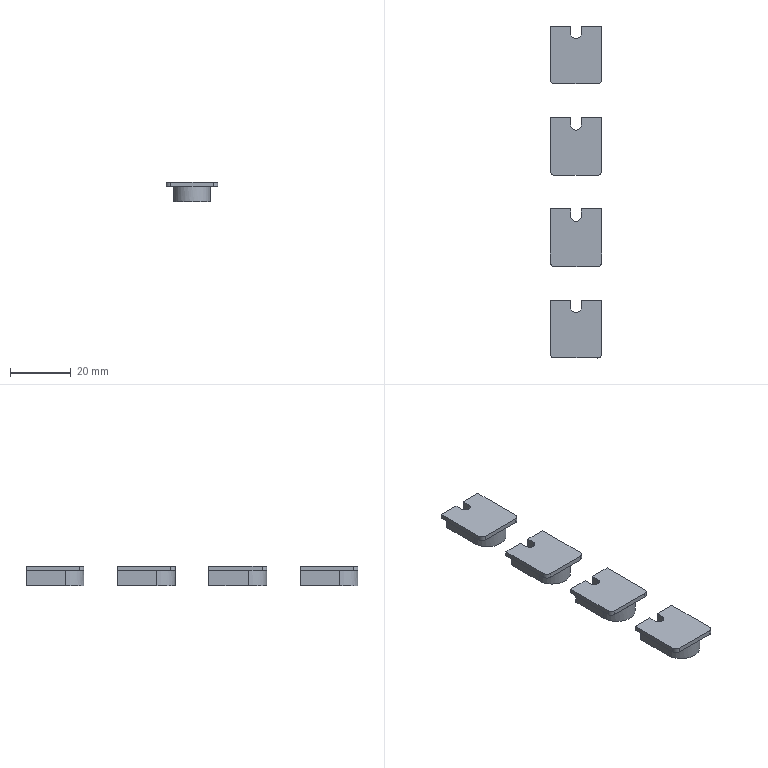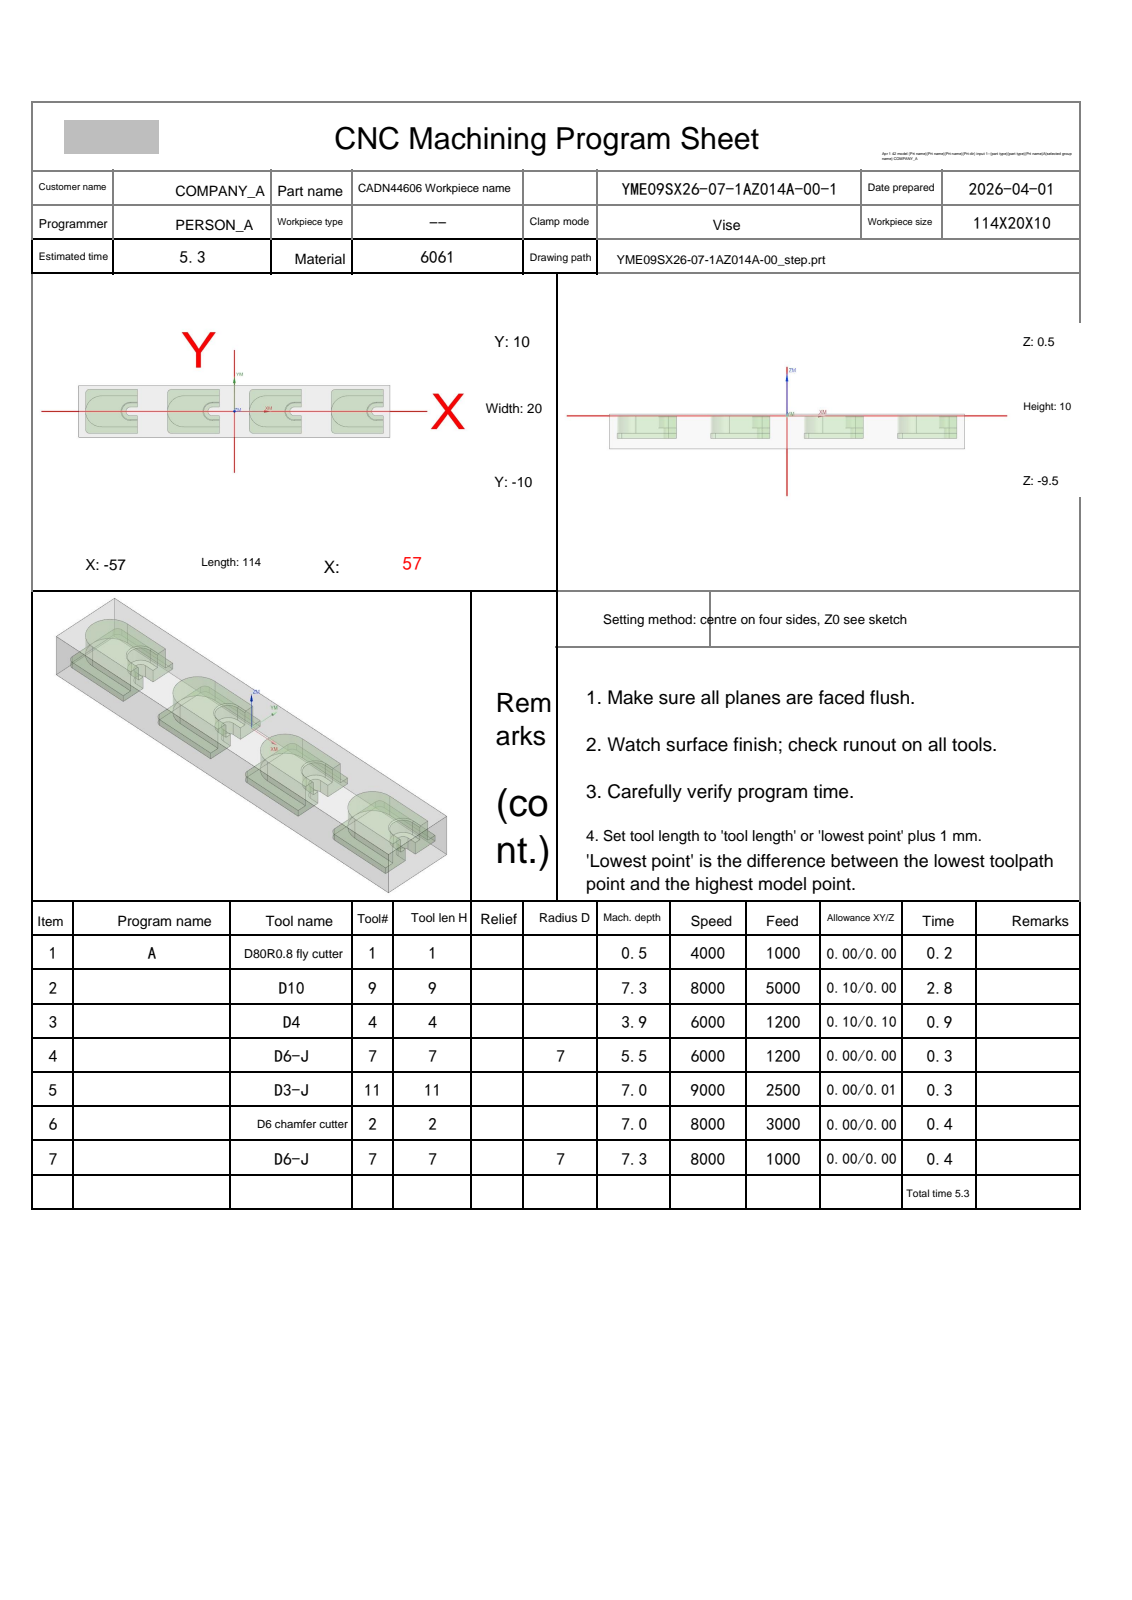NC program | NX | posted by the shop | part box 17.001 x 109 x 6.504 mm
Lines 2417 to 4321 of 4321, first 1691 of 1905 lines:
N5 T11 M06
(D3-J  D=3. R=0. H=11 ce=0.00 di=0.01)
G00 G90 G54 X-33.527 Y1.705 M03 S9000
G43 H11 Z20.
M08
Z-3.068
G01 X-33.532 Z-3.133 F2000.
X-33.547 Z-3.191
X-33.569 Y1.704 Z-3.243
X-33.598 Y1.703 Z-3.29
X-33.633 Y1.7 Z-3.332
X-33.673 Y1.696 Z-3.369
X-33.715 Y1.689 Z-3.401
X-33.758 Y1.68 Z-3.428
X-33.803 Y1.669 Z-3.451
X-33.846 Y1.654 Z-3.471
X-33.887 Y1.635 Z-3.486
X-33.925 Y1.613 Z-3.498
X-33.958 Y1.587 Z-3.508
X-33.985 Y1.555 Z-3.514
X-34.005 Y1.519 Z-3.517
X-34.017 Y1.477 Z-3.518
G02 X-35.501 Y.2 I-1.484 J.223 F2500.
G01 X-35.537
X-37.998
X-38.
G03 X-38.2 Y0.0 I0.0 J-.2
G01 X-38.13 Y-.152
X-38.097 Y-.186
X-38.053 Y-.203
X-38.005 Y-.2
X-35.489
G02 X-34.017 Y-1.477 I-.011 J-1.5
G01 X-34.002 Y-1.508 Z-3.519
X-33.974 Y-1.502 Z-3.523
X-33.936 Y-1.464 Z-3.529
X-33.89 Y-1.398 Z-3.537
X-33.84 Y-1.306 Z-3.547
X-33.787 Y-1.193 Z-3.558
X-33.735 Y-1.062 Z-3.57
X-33.687 Y-.918 Z-3.584
X-33.644 Y-.763 Z-3.598
X-33.588 Y-.467 Z-3.624
X-33.56 Y-.158 Z-3.651
Y.156 Z-3.679
X-33.588 Y.465 Z-3.706
X-33.644 Y.761 Z-3.732
X-33.687 Y.916 Z-3.746
X-33.735 Y1.061 Z-3.759
X-33.787 Y1.192 Z-3.772
X-33.84 Y1.305 Z-3.783
X-33.89 Y1.397 Z-3.792
X-33.936 Y1.464 Z-3.8
X-33.974 Y1.502 Z-3.806
X-34.002 Y1.508 Z-3.81
X-34.017 Y1.477 Z-3.811
G02 X-35.5 Y.2 I-1.483 J.223
G01 X-35.506
X-37.998
X-38.
G03 X-38.2 Y0.0 I0.0 J-.2
G01 X-38.13 Y-.152
X-38.097 Y-.186
X-38.053 Y-.203
X-38.005 Y-.2
X-35.489
G02 X-34.017 Y-1.477 I-.011 J-1.5
G01 X-34.002 Y-1.508 Z-3.813
X-33.974 Y-1.502 Z-3.816
X-33.936 Y-1.464 Z-3.822
X-33.89 Y-1.398 Z-3.83
X-33.84 Y-1.306 Z-3.84
X-33.787 Y-1.193 Z-3.851
X-33.735 Y-1.062 Z-3.864
X-33.687 Y-.918 Z-3.877
X-33.644 Y-.763 Z-3.891
X-33.588 Y-.467 Z-3.917
X-33.56 Y-.158 Z-3.944
Y.156 Z-3.972
X-33.588 Y.465 Z-3.999
X-33.644 Y.761 Z-4.025
X-33.687 Y.916 Z-4.039
X-33.735 Y1.061 Z-4.052
X-33.787 Y1.192 Z-4.065
X-33.84 Y1.305 Z-4.076
X-33.89 Y1.397 Z-4.086
X-33.936 Y1.464 Z-4.093
X-33.974 Y1.502 Z-4.099
X-34.002 Y1.508 Z-4.103
X-34.017 Y1.477 Z-4.105
G02 X-35.5 Y.2 I-1.483 J.223
G01 X-35.506
X-37.998
X-38.
G03 X-38.2 Y0.0 I0.0 J-.2
G01 X-38.13 Y-.152
X-38.097 Y-.186
X-38.053 Y-.203
X-38.005 Y-.2
X-35.489
G02 X-34.017 Y-1.477 I-.011 J-1.5
G01 X-34.002 Y-1.508 Z-4.106
X-33.974 Y-1.502 Z-4.11
X-33.936 Y-1.464 Z-4.116
X-33.89 Y-1.398 Z-4.124
X-33.84 Y-1.306 Z-4.133
X-33.787 Y-1.193 Z-4.144
X-33.735 Y-1.062 Z-4.157
X-33.687 Y-.918 Z-4.17
X-33.644 Y-.763 Z-4.184
X-33.588 Y-.467 Z-4.21
X-33.56 Y-.158 Z-4.237
Y.156 Z-4.265
X-33.588 Y.465 Z-4.292
X-33.644 Y.761 Z-4.318
X-33.687 Y.916 Z-4.332
X-33.735 Y1.061 Z-4.346
X-33.787 Y1.192 Z-4.358
X-33.84 Y1.305 Z-4.369
X-33.89 Y1.397 Z-4.379
X-33.936 Y1.464 Z-4.387
X-33.974 Y1.502 Z-4.393
X-34.002 Y1.508 Z-4.396
X-34.017 Y1.477 Z-4.398
G02 X-35.5 Y.2 I-1.483 J.223
G01 X-35.506
X-37.998
X-38.
G03 X-38.2 Y0.0 I0.0 J-.2
G01 X-38.13 Y-.152
X-38.097 Y-.186
X-38.053 Y-.203
X-38.005 Y-.2
X-35.489
G02 X-34.017 Y-1.477 I-.011 J-1.5
G01 X-34.002 Y-1.508 Z-4.399
X-33.974 Y-1.502 Z-4.403
X-33.936 Y-1.464 Z-4.409
X-33.89 Y-1.398 Z-4.417
X-33.84 Y-1.306 Z-4.426
X-33.787 Y-1.193 Z-4.438
X-33.735 Y-1.062 Z-4.45
X-33.687 Y-.918 Z-4.463
X-33.644 Y-.763 Z-4.477
X-33.588 Y-.467 Z-4.503
X-33.56 Y-.158 Z-4.531
Y.156 Z-4.558
X-33.588 Y.465 Z-4.585
X-33.644 Y.761 Z-4.612
X-33.687 Y.916 Z-4.625
X-33.735 Y1.061 Z-4.639
X-33.787 Y1.192 Z-4.651
X-33.84 Y1.305 Z-4.662
X-33.89 Y1.397 Z-4.672
X-33.936 Y1.464 Z-4.68
X-33.974 Y1.502 Z-4.686
X-34.002 Y1.508 Z-4.69
X-34.017 Y1.477 Z-4.691
G02 X-35.5 Y.2 I-1.483 J.223
G01 X-35.506
X-37.998
X-38.
G03 X-38.2 Y0.0 I0.0 J-.2
G01 X-38.13 Y-.152
X-38.097 Y-.186
X-38.053 Y-.203
X-38.005 Y-.2
X-35.489
G02 X-34.017 Y-1.477 I-.011 J-1.5
G01 X-34.002 Y-1.508 Z-4.692
X-33.974 Y-1.502 Z-4.696
X-33.936 Y-1.464 Z-4.702
X-33.89 Y-1.398 Z-4.71
X-33.84 Y-1.306 Z-4.72
X-33.787 Y-1.193 Z-4.731
X-33.735 Y-1.062 Z-4.743
X-33.687 Y-.918 Z-4.756
X-33.644 Y-.763 Z-4.77
X-33.588 Y-.467 Z-4.797
X-33.56 Y-.158 Z-4.824
Y.156 Z-4.851
X-33.588 Y.465 Z-4.878
X-33.644 Y.761 Z-4.905
X-33.687 Y.916 Z-4.919
X-33.735 Y1.061 Z-4.932
X-33.787 Y1.192 Z-4.944
X-33.84 Y1.305 Z-4.955
X-33.89 Y1.397 Z-4.965
X-33.936 Y1.464 Z-4.973
X-33.974 Y1.502 Z-4.979
X-34.002 Y1.508 Z-4.983
X-34.017 Y1.477 Z-4.984
G02 X-35.5 Y.2 I-1.483 J.223
G01 X-35.506
X-37.998
X-38.
G03 X-38.2 Y0.0 I0.0 J-.2
G01 X-38.13 Y-.152
X-38.097 Y-.186
X-38.053 Y-.203
X-38.005 Y-.2
X-35.489
G02 X-34.017 Y-1.477 I-.011 J-1.5
G01 X-34.002 Y-1.508 Z-4.985
X-33.974 Y-1.502 Z-4.989
X-33.936 Y-1.464 Z-4.995
X-33.89 Y-1.398 Z-5.003
X-33.84 Y-1.306 Z-5.013
X-33.787 Y-1.193 Z-5.024
X-33.735 Y-1.062 Z-5.036
X-33.687 Y-.918 Z-5.05
X-33.644 Y-.763 Z-5.063
X-33.588 Y-.467 Z-5.09
X-33.56 Y-.158 Z-5.117
Y.156 Z-5.144
X-33.588 Y.465 Z-5.172
X-33.644 Y.761 Z-5.198
X-33.687 Y.916 Z-5.212
X-33.735 Y1.061 Z-5.225
X-33.787 Y1.192 Z-5.237
X-33.84 Y1.305 Z-5.249
X-33.89 Y1.397 Z-5.258
X-33.936 Y1.464 Z-5.266
X-33.974 Y1.502 Z-5.272
X-34.002 Y1.508 Z-5.276
X-34.017 Y1.477 Z-5.277
G02 X-35.5 Y.2 I-1.483 J.223
G01 X-35.506
X-37.998
X-38.
G03 X-38.2 Y0.0 I0.0 J-.2
G01 X-38.13 Y-.152
X-38.097 Y-.186
X-38.053 Y-.203
X-38.005 Y-.2
X-35.489
G02 X-34.017 Y-1.477 I-.011 J-1.5
G01 X-34.002 Y-1.508 Z-5.279
X-33.974 Y-1.502 Z-5.282
X-33.936 Y-1.464 Z-5.288
X-33.89 Y-1.398 Z-5.296
X-33.84 Y-1.306 Z-5.306
X-33.787 Y-1.193 Z-5.317
X-33.735 Y-1.062 Z-5.329
X-33.687 Y-.918 Z-5.343
X-33.644 Y-.763 Z-5.357
X-33.588 Y-.467 Z-5.383
X-33.56 Y-.158 Z-5.41
Y.156 Z-5.438
X-33.588 Y.465 Z-5.465
X-33.644 Y.761 Z-5.491
X-33.687 Y.916 Z-5.505
X-33.735 Y1.061 Z-5.518
X-33.787 Y1.192 Z-5.531
X-33.84 Y1.305 Z-5.542
X-33.89 Y1.397 Z-5.551
X-33.936 Y1.464 Z-5.559
X-33.974 Y1.502 Z-5.565
X-34.002 Y1.508 Z-5.569
X-34.017 Y1.477 Z-5.57
G02 X-35.5 Y.2 I-1.483 J.223
G01 X-35.506
X-37.998
X-38.
G03 X-38.2 Y0.0 I0.0 J-.2
G01 X-38.13 Y-.152
X-38.097 Y-.186
X-38.053 Y-.203
X-38.005 Y-.2
X-35.489
G02 X-34.017 Y-1.477 I-.011 J-1.5
G01 X-34.002 Y-1.508 Z-5.572
X-33.974 Y-1.502 Z-5.576
X-33.936 Y-1.464 Z-5.582
X-33.89 Y-1.398 Z-5.589
X-33.84 Y-1.306 Z-5.599
X-33.787 Y-1.193 Z-5.61
X-33.735 Y-1.062 Z-5.623
X-33.687 Y-.918 Z-5.636
X-33.644 Y-.763 Z-5.65
X-33.588 Y-.467 Z-5.676
X-33.56 Y-.158 Z-5.703
Y.156 Z-5.731
X-33.588 Y.465 Z-5.758
X-33.644 Y.761 Z-5.784
X-33.687 Y.916 Z-5.798
X-33.735 Y1.061 Z-5.811
X-33.787 Y1.192 Z-5.824
X-33.84 Y1.305 Z-5.835
X-33.89 Y1.397 Z-5.845
X-33.936 Y1.464 Z-5.853
X-33.974 Y1.502 Z-5.859
X-34.002 Y1.508 Z-5.862
X-34.017 Y1.477 Z-5.864
G02 X-35.5 Y.2 I-1.483 J.223
G01 X-35.506
X-37.998
X-38.
G03 X-38.2 Y0.0 I0.0 J-.2
G01 X-38.13 Y-.152
X-38.097 Y-.186
X-38.053 Y-.203
X-38.005 Y-.2
X-35.489
G02 X-34.017 Y-1.477 I-.011 J-1.5
G01 X-34.002 Y-1.508 Z-5.865
X-33.974 Y-1.502 Z-5.869
X-33.936 Y-1.464 Z-5.875
X-33.89 Y-1.398 Z-5.883
X-33.84 Y-1.306 Z-5.892
X-33.787 Y-1.193 Z-5.903
X-33.735 Y-1.062 Z-5.916
X-33.687 Y-.918 Z-5.929
X-33.644 Y-.763 Z-5.943
X-33.588 Y-.467 Z-5.969
X-33.56 Y-.158 Z-5.996
Y.156 Z-6.024
X-33.588 Y.465 Z-6.051
X-33.644 Y.761 Z-6.077
X-33.687 Y.916 Z-6.091
X-33.735 Y1.061 Z-6.105
X-33.787 Y1.192 Z-6.117
X-33.84 Y1.305 Z-6.128
X-33.89 Y1.397 Z-6.138
X-33.936 Y1.464 Z-6.146
X-33.974 Y1.502 Z-6.152
X-34.002 Y1.508 Z-6.156
X-34.017 Y1.477 Z-6.157
G02 X-35.5 Y.2 I-1.483 J.223
G01 X-35.506
X-37.998
X-38.
G03 X-38.2 Y0.0 I0.0 J-.2
G01 X-38.13 Y-.152
X-38.097 Y-.186
X-38.053 Y-.203
X-38.005 Y-.2
X-35.489
G02 X-34.017 Y-1.477 I-.011 J-1.5
G01 X-34.002 Y-1.508 Z-6.158
X-33.974 Y-1.502 Z-6.162
X-33.936 Y-1.464 Z-6.168
X-33.89 Y-1.398 Z-6.176
X-33.84 Y-1.306 Z-6.186
X-33.787 Y-1.193 Z-6.197
X-33.735 Y-1.062 Z-6.209
X-33.687 Y-.918 Z-6.222
X-33.644 Y-.763 Z-6.236
X-33.588 Y-.467 Z-6.263
X-33.56 Y-.158 Z-6.29
Y.156 Z-6.317
X-33.588 Y.465 Z-6.344
X-33.644 Y.761 Z-6.371
X-33.687 Y.916 Z-6.385
X-33.735 Y1.061 Z-6.398
X-33.787 Y1.192 Z-6.41
X-33.84 Y1.305 Z-6.421
X-33.89 Y1.397 Z-6.431
X-33.936 Y1.464 Z-6.439
X-33.974 Y1.502 Z-6.445
X-34.002 Y1.508 Z-6.449
X-34.017 Y1.477 Z-6.45
G02 X-35.5 Y.2 I-1.483 J.223
G01 X-35.506
X-37.998
X-38.
G03 X-38.2 Y0.0 I0.0 J-.2
G01 X-38.13 Y-.152
X-38.097 Y-.186
X-38.053 Y-.203
X-38.005 Y-.2
X-35.489
G02 X-34.017 Y-1.477 I-.011 J-1.5
G01 X-33.986 Y-1.515 Z-6.449
X-33.947 Y-1.546 Z-6.445
X-33.902 Y-1.573 Z-6.438
X-33.852 Y-1.596 Z-6.427
X-33.799 Y-1.614 Z-6.413
X-33.744 Y-1.628 Z-6.395
X-33.689 Y-1.64 Z-6.373
X-33.634 Y-1.648 Z-6.346
X-33.582 Y-1.654 Z-6.314
X-33.535 Y-1.658 Z-6.277
X-33.492 Y-1.66 Z-6.234
X-33.456 Y-1.661 Z-6.185
X-33.429 Z-6.13
X-33.412 Z-6.068
X-33.406 Z-6.
G00 Z20.
X-3.527 Y1.705
Z-3.068
G01 X-3.532 Z-3.133 F2000.
X-3.547 Z-3.191
X-3.569 Y1.704 Z-3.243
X-3.598 Y1.703 Z-3.29
X-3.633 Y1.7 Z-3.332
X-3.673 Y1.696 Z-3.369
X-3.715 Y1.689 Z-3.401
X-3.758 Y1.68 Z-3.428
X-3.803 Y1.669 Z-3.451
X-3.846 Y1.654 Z-3.471
X-3.887 Y1.635 Z-3.486
X-3.925 Y1.613 Z-3.498
X-3.958 Y1.587 Z-3.508
X-3.985 Y1.555 Z-3.514
X-4.005 Y1.519 Z-3.517
X-4.017 Y1.477 Z-3.518
G02 X-5.493 Y.2 I-1.483 J.223 F2500.
G01 X-7.998
X-8.
G03 X-8.2 Y0.0 I0.0 J-.2
X-8. Y-.2 I.2 J0.0
G01 X-7.998
X-5.489
G02 X-4.017 Y-1.477 I-.011 J-1.5
G01 X-4.002 Y-1.507 Z-3.519
X-3.975 Y-1.499 Z-3.523
X-3.937 Y-1.457 Z-3.529
X-3.892 Y-1.386 Z-3.537
X-3.842 Y-1.289 Z-3.547
X-3.791 Y-1.171 Z-3.558
X-3.739 Y-1.035 Z-3.57
X-3.691 Y-.886 Z-3.584
X-3.649 Y-.728 Z-3.598
X-3.593 Y-.43 Z-3.624
X-3.565 Y-.122 Z-3.651
X-3.564 Y.187 Z-3.679
X-3.591 Y.491 Z-3.706
X-3.647 Y.781 Z-3.732
X-3.689 Y.932 Z-3.746
X-3.737 Y1.074 Z-3.759
X-3.789 Y1.202 Z-3.772
X-3.841 Y1.312 Z-3.783
X-3.891 Y1.402 Z-3.792
X-3.936 Y1.467 Z-3.8
X-3.974 Y1.503 Z-3.806
X-4.002 Y1.508 Z-3.81
X-4.017 Y1.477 Z-3.811
G02 X-5.493 Y.2 I-1.483 J.223
G01 X-7.998
X-8.
G03 X-8.2 Y0.0 I0.0 J-.2
X-8. Y-.2 I.2 J0.0
G01 X-7.998
X-5.489
G02 X-4.017 Y-1.477 I-.011 J-1.5
G01 X-4.002 Y-1.507 Z-3.813
X-3.975 Y-1.499 Z-3.816
X-3.937 Y-1.457 Z-3.822
X-3.892 Y-1.386 Z-3.83
X-3.842 Y-1.289 Z-3.84
X-3.791 Y-1.171 Z-3.851
X-3.739 Y-1.035 Z-3.864
X-3.691 Y-.886 Z-3.877
X-3.649 Y-.728 Z-3.891
X-3.593 Y-.43 Z-3.917
X-3.565 Y-.122 Z-3.944
X-3.564 Y.187 Z-3.972
X-3.591 Y.491 Z-3.999
X-3.647 Y.781 Z-4.025
X-3.689 Y.932 Z-4.039
X-3.737 Y1.074 Z-4.052
X-3.789 Y1.202 Z-4.065
X-3.841 Y1.312 Z-4.076
X-3.891 Y1.402 Z-4.086
X-3.936 Y1.467 Z-4.093
X-3.974 Y1.503 Z-4.099
X-4.002 Y1.508 Z-4.103
X-4.017 Y1.477 Z-4.105
G02 X-5.493 Y.2 I-1.483 J.223
G01 X-7.998
X-8.
G03 X-8.2 Y0.0 I0.0 J-.2
X-8. Y-.2 I.2 J0.0
G01 X-7.998
X-5.489
G02 X-4.017 Y-1.477 I-.011 J-1.5
G01 X-4.002 Y-1.507 Z-4.106
X-3.975 Y-1.499 Z-4.11
X-3.937 Y-1.457 Z-4.116
X-3.892 Y-1.386 Z-4.124
X-3.842 Y-1.289 Z-4.133
X-3.791 Y-1.171 Z-4.144
X-3.739 Y-1.035 Z-4.157
X-3.691 Y-.886 Z-4.17
X-3.649 Y-.728 Z-4.184
X-3.593 Y-.43 Z-4.21
X-3.565 Y-.122 Z-4.237
X-3.564 Y.187 Z-4.265
X-3.591 Y.491 Z-4.292
X-3.647 Y.781 Z-4.318
X-3.689 Y.932 Z-4.332
X-3.737 Y1.074 Z-4.346
X-3.789 Y1.202 Z-4.358
X-3.841 Y1.312 Z-4.369
X-3.891 Y1.402 Z-4.379
X-3.936 Y1.467 Z-4.387
X-3.974 Y1.503 Z-4.393
X-4.002 Y1.508 Z-4.396
X-4.017 Y1.477 Z-4.398
G02 X-5.493 Y.2 I-1.483 J.223
G01 X-7.998
X-8.
G03 X-8.2 Y0.0 I0.0 J-.2
X-8. Y-.2 I.2 J0.0
G01 X-7.998
X-5.489
G02 X-4.017 Y-1.477 I-.011 J-1.5
G01 X-4.002 Y-1.507 Z-4.399
X-3.975 Y-1.499 Z-4.403
X-3.937 Y-1.457 Z-4.409
X-3.892 Y-1.386 Z-4.417
X-3.842 Y-1.289 Z-4.426
X-3.791 Y-1.171 Z-4.438
X-3.739 Y-1.035 Z-4.45
X-3.691 Y-.886 Z-4.463
X-3.649 Y-.728 Z-4.477
X-3.593 Y-.43 Z-4.503
X-3.565 Y-.122 Z-4.531
X-3.564 Y.187 Z-4.558
X-3.591 Y.491 Z-4.585
X-3.647 Y.781 Z-4.612
X-3.689 Y.932 Z-4.625
X-3.737 Y1.074 Z-4.639
X-3.789 Y1.202 Z-4.651
X-3.841 Y1.312 Z-4.662
X-3.891 Y1.402 Z-4.672
X-3.936 Y1.467 Z-4.68
X-3.974 Y1.503 Z-4.686
X-4.002 Y1.508 Z-4.69
X-4.017 Y1.477 Z-4.691
G02 X-5.493 Y.2 I-1.483 J.223
G01 X-7.998
X-8.
G03 X-8.2 Y0.0 I0.0 J-.2
X-8. Y-.2 I.2 J0.0
G01 X-7.998
X-5.489
G02 X-4.017 Y-1.477 I-.011 J-1.5
G01 X-4.002 Y-1.507 Z-4.692
X-3.975 Y-1.499 Z-4.696
X-3.937 Y-1.457 Z-4.702
X-3.892 Y-1.386 Z-4.71
X-3.842 Y-1.289 Z-4.72
X-3.791 Y-1.171 Z-4.731
X-3.739 Y-1.035 Z-4.743
X-3.691 Y-.886 Z-4.756
X-3.649 Y-.728 Z-4.77
X-3.593 Y-.43 Z-4.797
X-3.565 Y-.122 Z-4.824
X-3.564 Y.187 Z-4.851
X-3.591 Y.491 Z-4.878
X-3.647 Y.781 Z-4.905
X-3.689 Y.932 Z-4.919
X-3.737 Y1.074 Z-4.932
X-3.789 Y1.202 Z-4.944
X-3.841 Y1.312 Z-4.955
X-3.891 Y1.402 Z-4.965
X-3.936 Y1.467 Z-4.973
X-3.974 Y1.503 Z-4.979
X-4.002 Y1.508 Z-4.983
X-4.017 Y1.477 Z-4.984
G02 X-5.493 Y.2 I-1.483 J.223
G01 X-7.998
X-8.
G03 X-8.2 Y0.0 I0.0 J-.2
X-8. Y-.2 I.2 J0.0
G01 X-7.998
X-5.489
G02 X-4.017 Y-1.477 I-.011 J-1.5
G01 X-4.002 Y-1.507 Z-4.985
X-3.975 Y-1.499 Z-4.989
X-3.937 Y-1.457 Z-4.995
X-3.892 Y-1.386 Z-5.003
X-3.842 Y-1.289 Z-5.013
X-3.791 Y-1.171 Z-5.024
X-3.739 Y-1.035 Z-5.036
X-3.691 Y-.886 Z-5.05
X-3.649 Y-.728 Z-5.063
X-3.593 Y-.43 Z-5.09
X-3.565 Y-.122 Z-5.117
X-3.564 Y.187 Z-5.144
X-3.591 Y.491 Z-5.172
X-3.647 Y.781 Z-5.198
X-3.689 Y.932 Z-5.212
X-3.737 Y1.074 Z-5.225
X-3.789 Y1.202 Z-5.237
X-3.841 Y1.312 Z-5.249
X-3.891 Y1.402 Z-5.258
X-3.936 Y1.467 Z-5.266
X-3.974 Y1.503 Z-5.272
X-4.002 Y1.508 Z-5.276
X-4.017 Y1.477 Z-5.277
G02 X-5.493 Y.2 I-1.483 J.223
G01 X-7.998
X-8.
G03 X-8.2 Y0.0 I0.0 J-.2
X-8. Y-.2 I.2 J0.0
G01 X-7.998
X-5.489
G02 X-4.017 Y-1.477 I-.011 J-1.5
G01 X-4.002 Y-1.507 Z-5.279
X-3.975 Y-1.499 Z-5.282
X-3.937 Y-1.457 Z-5.288
X-3.892 Y-1.386 Z-5.296
X-3.842 Y-1.289 Z-5.306
X-3.791 Y-1.171 Z-5.317
X-3.739 Y-1.035 Z-5.329
X-3.691 Y-.886 Z-5.343
X-3.649 Y-.728 Z-5.357
X-3.593 Y-.43 Z-5.383
X-3.565 Y-.122 Z-5.41
X-3.564 Y.187 Z-5.438
X-3.591 Y.491 Z-5.465
X-3.647 Y.781 Z-5.491
X-3.689 Y.932 Z-5.505
X-3.737 Y1.074 Z-5.518
X-3.789 Y1.202 Z-5.531
X-3.841 Y1.312 Z-5.542
X-3.891 Y1.402 Z-5.551
X-3.936 Y1.467 Z-5.559
X-3.974 Y1.503 Z-5.565
X-4.002 Y1.508 Z-5.569
X-4.017 Y1.477 Z-5.57
G02 X-5.493 Y.2 I-1.483 J.223
G01 X-7.998
X-8.
G03 X-8.2 Y0.0 I0.0 J-.2
X-8. Y-.2 I.2 J0.0
G01 X-7.998
X-5.489
G02 X-4.017 Y-1.477 I-.011 J-1.5
G01 X-4.002 Y-1.507 Z-5.572
X-3.975 Y-1.499 Z-5.576
X-3.937 Y-1.457 Z-5.582
X-3.892 Y-1.386 Z-5.589
X-3.842 Y-1.289 Z-5.599
X-3.791 Y-1.171 Z-5.61
X-3.739 Y-1.035 Z-5.623
X-3.691 Y-.886 Z-5.636
X-3.649 Y-.728 Z-5.65
X-3.593 Y-.43 Z-5.676
X-3.565 Y-.122 Z-5.703
X-3.564 Y.187 Z-5.731
X-3.591 Y.491 Z-5.758
X-3.647 Y.781 Z-5.784
X-3.689 Y.932 Z-5.798
X-3.737 Y1.074 Z-5.811
X-3.789 Y1.202 Z-5.824
X-3.841 Y1.312 Z-5.835
X-3.891 Y1.402 Z-5.845
X-3.936 Y1.467 Z-5.853
X-3.974 Y1.503 Z-5.859
X-4.002 Y1.508 Z-5.862
X-4.017 Y1.477 Z-5.864
G02 X-5.493 Y.2 I-1.483 J.223
G01 X-7.998
X-8.
G03 X-8.2 Y0.0 I0.0 J-.2
X-8. Y-.2 I.2 J0.0
G01 X-7.998
X-5.489
G02 X-4.017 Y-1.477 I-.011 J-1.5
G01 X-4.002 Y-1.507 Z-5.865
X-3.975 Y-1.499 Z-5.869
X-3.937 Y-1.457 Z-5.875
X-3.892 Y-1.386 Z-5.883
X-3.842 Y-1.289 Z-5.892
X-3.791 Y-1.171 Z-5.903
X-3.739 Y-1.035 Z-5.916
X-3.691 Y-.886 Z-5.929
X-3.649 Y-.728 Z-5.943
X-3.593 Y-.43 Z-5.969
X-3.565 Y-.122 Z-5.996
X-3.564 Y.187 Z-6.024
X-3.591 Y.491 Z-6.051
X-3.647 Y.781 Z-6.077
X-3.689 Y.932 Z-6.091
X-3.737 Y1.074 Z-6.105
X-3.789 Y1.202 Z-6.117
X-3.841 Y1.312 Z-6.128
X-3.891 Y1.402 Z-6.138
X-3.936 Y1.467 Z-6.146
X-3.974 Y1.503 Z-6.152
X-4.002 Y1.508 Z-6.156
X-4.017 Y1.477 Z-6.157
G02 X-5.493 Y.2 I-1.483 J.223
G01 X-7.998
X-8.
G03 X-8.2 Y0.0 I0.0 J-.2
X-8. Y-.2 I.2 J0.0
G01 X-7.998
X-5.489
G02 X-4.017 Y-1.477 I-.011 J-1.5
G01 X-4.002 Y-1.507 Z-6.158
X-3.975 Y-1.499 Z-6.162
X-3.937 Y-1.457 Z-6.168
X-3.892 Y-1.386 Z-6.176
X-3.842 Y-1.289 Z-6.186
X-3.791 Y-1.171 Z-6.197
X-3.739 Y-1.035 Z-6.209
X-3.691 Y-.886 Z-6.222
X-3.649 Y-.728 Z-6.236
X-3.593 Y-.43 Z-6.263
X-3.565 Y-.122 Z-6.29
X-3.564 Y.187 Z-6.317
X-3.591 Y.491 Z-6.344
X-3.647 Y.781 Z-6.371
X-3.689 Y.932 Z-6.385
X-3.737 Y1.074 Z-6.398
X-3.789 Y1.202 Z-6.41
X-3.841 Y1.312 Z-6.421
X-3.891 Y1.402 Z-6.431
X-3.936 Y1.467 Z-6.439
X-3.974 Y1.503 Z-6.445
X-4.002 Y1.508 Z-6.449
X-4.017 Y1.477 Z-6.45
G02 X-5.493 Y.2 I-1.483 J.223
G01 X-7.998
X-8.
G03 X-8.2 Y0.0 I0.0 J-.2
X-8. Y-.2 I.2 J0.0
G01 X-7.998
X-5.489
G02 X-4.017 Y-1.477 I-.011 J-1.5
G01 X-3.986 Y-1.514 Z-6.449
X-3.948 Y-1.543 Z-6.445
X-3.903 Y-1.566 Z-6.438
X-3.854 Y-1.583 Z-6.427
X-3.802 Y-1.595 Z-6.413
X-3.748 Y-1.603 Z-6.395
X-3.693 Y-1.607 Z-6.373
X-3.64 Y-1.608 Z-6.346
X-3.589 Y-1.607 Z-6.314
X-3.542 Y-1.604 Z-6.277
X-3.501 Y-1.6 Z-6.234
X-3.466 Y-1.596 Z-6.185
X-3.439 Y-1.592 Z-6.13
X-3.422 Y-1.589 Z-6.068
X-3.416 Y-1.588 Z-6.
G00 Z20.
X26.473 Y1.705
Z-3.068
G01 X26.468 Z-3.133 F2000.
X26.453 Z-3.191
X26.431 Y1.704 Z-3.243
X26.402 Y1.703 Z-3.29
X26.367 Y1.7 Z-3.332
X26.327 Y1.696 Z-3.369
X26.285 Y1.689 Z-3.401
X26.242 Y1.68 Z-3.428
X26.197 Y1.669 Z-3.451
X26.154 Y1.654 Z-3.471
X26.113 Y1.635 Z-3.486
X26.075 Y1.613 Z-3.498
X26.042 Y1.587 Z-3.508
X26.015 Y1.555 Z-3.514
X25.995 Y1.519 Z-3.517
X25.983 Y1.477 Z-3.518
G02 X24.507 Y.2 I-1.483 J.223 F2500.
G01 X22.002
X22.
G03 X21.8 Y0.0 I0.0 J-.2
X22. Y-.2 I.2 J0.0
G01 X22.002
X24.511
G02 X25.983 Y-1.477 I-.011 J-1.5
G01 X25.998 Y-1.507 Z-3.519
X26.025 Y-1.499 Z-3.523
X26.063 Y-1.457 Z-3.529
X26.108 Y-1.386 Z-3.537
X26.158 Y-1.289 Z-3.547
X26.209 Y-1.171 Z-3.558
X26.261 Y-1.035 Z-3.57
X26.309 Y-.886 Z-3.584
X26.351 Y-.728 Z-3.598
X26.407 Y-.43 Z-3.624
X26.435 Y-.122 Z-3.651
X26.436 Y.187 Z-3.679
X26.409 Y.491 Z-3.706
X26.353 Y.781 Z-3.732
X26.311 Y.932 Z-3.746
X26.263 Y1.074 Z-3.759
X26.211 Y1.202 Z-3.772
X26.159 Y1.312 Z-3.783
X26.109 Y1.402 Z-3.792
X26.064 Y1.467 Z-3.8
X26.026 Y1.503 Z-3.806
X25.998 Y1.508 Z-3.81
X25.983 Y1.477 Z-3.811
G02 X24.507 Y.2 I-1.483 J.223
G01 X22.002
X22.
G03 X21.8 Y0.0 I0.0 J-.2
X22. Y-.2 I.2 J0.0
G01 X22.002
X24.511
G02 X25.983 Y-1.477 I-.011 J-1.5
G01 X25.998 Y-1.507 Z-3.813
X26.025 Y-1.499 Z-3.816
X26.063 Y-1.457 Z-3.822
X26.108 Y-1.386 Z-3.83
X26.158 Y-1.289 Z-3.84
X26.209 Y-1.171 Z-3.851
X26.261 Y-1.035 Z-3.864
X26.309 Y-.886 Z-3.877
X26.351 Y-.728 Z-3.891
X26.407 Y-.43 Z-3.917
X26.435 Y-.122 Z-3.944
X26.436 Y.187 Z-3.972
X26.409 Y.491 Z-3.999
X26.353 Y.781 Z-4.025
X26.311 Y.932 Z-4.039
X26.263 Y1.074 Z-4.052
X26.211 Y1.202 Z-4.065
X26.159 Y1.312 Z-4.076
X26.109 Y1.402 Z-4.086
X26.064 Y1.467 Z-4.093
X26.026 Y1.503 Z-4.099
X25.998 Y1.508 Z-4.103
X25.983 Y1.477 Z-4.105
G02 X24.507 Y.2 I-1.483 J.223
G01 X22.002
X22.
G03 X21.8 Y0.0 I0.0 J-.2
X22. Y-.2 I.2 J0.0
G01 X22.002
X24.511
G02 X25.983 Y-1.477 I-.011 J-1.5
G01 X25.998 Y-1.507 Z-4.106
X26.025 Y-1.499 Z-4.11
X26.063 Y-1.457 Z-4.116
X26.108 Y-1.386 Z-4.124
X26.158 Y-1.289 Z-4.133
X26.209 Y-1.171 Z-4.144
X26.261 Y-1.035 Z-4.157
X26.309 Y-.886 Z-4.17
X26.351 Y-.728 Z-4.184
X26.407 Y-.43 Z-4.21
X26.435 Y-.122 Z-4.237
X26.436 Y.187 Z-4.265
X26.409 Y.491 Z-4.292
X26.353 Y.781 Z-4.318
X26.311 Y.932 Z-4.332
X26.263 Y1.074 Z-4.346
X26.211 Y1.202 Z-4.358
X26.159 Y1.312 Z-4.369
X26.109 Y1.402 Z-4.379
X26.064 Y1.467 Z-4.387
X26.026 Y1.503 Z-4.393
X25.998 Y1.508 Z-4.396
X25.983 Y1.477 Z-4.398
G02 X24.507 Y.2 I-1.483 J.223
G01 X22.002
X22.
G03 X21.8 Y0.0 I0.0 J-.2
X22. Y-.2 I.2 J0.0
G01 X22.002
X24.511
G02 X25.983 Y-1.477 I-.011 J-1.5
G01 X25.998 Y-1.507 Z-4.399
X26.025 Y-1.499 Z-4.403
X26.063 Y-1.457 Z-4.409
X26.108 Y-1.386 Z-4.417
X26.158 Y-1.289 Z-4.426
X26.209 Y-1.171 Z-4.438
X26.261 Y-1.035 Z-4.45
X26.309 Y-.886 Z-4.463
X26.351 Y-.728 Z-4.477
X26.407 Y-.43 Z-4.503
X26.435 Y-.122 Z-4.531
X26.436 Y.187 Z-4.558
X26.409 Y.491 Z-4.585
X26.353 Y.781 Z-4.612
X26.311 Y.932 Z-4.625
X26.263 Y1.074 Z-4.639
X26.211 Y1.202 Z-4.651
X26.159 Y1.312 Z-4.662
X26.109 Y1.402 Z-4.672
X26.064 Y1.467 Z-4.68
X26.026 Y1.503 Z-4.686
X25.998 Y1.508 Z-4.69
X25.983 Y1.477 Z-4.691
G02 X24.507 Y.2 I-1.483 J.223
G01 X22.002
X22.
G03 X21.8 Y0.0 I0.0 J-.2
X22. Y-.2 I.2 J0.0
G01 X22.002
X24.511
G02 X25.983 Y-1.477 I-.011 J-1.5
G01 X25.998 Y-1.507 Z-4.692
X26.025 Y-1.499 Z-4.696
X26.063 Y-1.457 Z-4.702
X26.108 Y-1.386 Z-4.71
X26.158 Y-1.289 Z-4.72
X26.209 Y-1.171 Z-4.731
X26.261 Y-1.035 Z-4.743
X26.309 Y-.886 Z-4.756
X26.351 Y-.728 Z-4.77
X26.407 Y-.43 Z-4.797
X26.435 Y-.122 Z-4.824
X26.436 Y.187 Z-4.851
X26.409 Y.491 Z-4.878
X26.353 Y.781 Z-4.905
X26.311 Y.932 Z-4.919
X26.263 Y1.074 Z-4.932
X26.211 Y1.202 Z-4.944
X26.159 Y1.312 Z-4.955
X26.109 Y1.402 Z-4.965
X26.064 Y1.467 Z-4.973
X26.026 Y1.503 Z-4.979
X25.998 Y1.508 Z-4.983
X25.983 Y1.477 Z-4.984
G02 X24.507 Y.2 I-1.483 J.223
G01 X22.002
X22.
G03 X21.8 Y0.0 I0.0 J-.2
X22. Y-.2 I.2 J0.0
G01 X22.002
X24.511
G02 X25.983 Y-1.477 I-.011 J-1.5
G01 X25.998 Y-1.507 Z-4.985
X26.025 Y-1.499 Z-4.989
X26.063 Y-1.457 Z-4.995
X26.108 Y-1.386 Z-5.003
X26.158 Y-1.289 Z-5.013
X26.209 Y-1.171 Z-5.024
X26.261 Y-1.035 Z-5.036
X26.309 Y-.886 Z-5.05
X26.351 Y-.728 Z-5.063
X26.407 Y-.43 Z-5.09
X26.435 Y-.122 Z-5.117
X26.436 Y.187 Z-5.144
X26.409 Y.491 Z-5.172
X26.353 Y.781 Z-5.198
X26.311 Y.932 Z-5.212
X26.263 Y1.074 Z-5.225
X26.211 Y1.202 Z-5.237
X26.159 Y1.312 Z-5.249
X26.109 Y1.402 Z-5.258
X26.064 Y1.467 Z-5.266
X26.026 Y1.503 Z-5.272
X25.998 Y1.508 Z-5.276
X25.983 Y1.477 Z-5.277
G02 X24.507 Y.2 I-1.483 J.223
G01 X22.002
X22.
G03 X21.8 Y0.0 I0.0 J-.2
X22. Y-.2 I.2 J0.0
G01 X22.002
X24.511
G02 X25.983 Y-1.477 I-.011 J-1.5
G01 X25.998 Y-1.507 Z-5.279
X26.025 Y-1.499 Z-5.282
X26.063 Y-1.457 Z-5.288
X26.108 Y-1.386 Z-5.296
X26.158 Y-1.289 Z-5.306
X26.209 Y-1.171 Z-5.317
X26.261 Y-1.035 Z-5.329
X26.309 Y-.886 Z-5.343
X26.351 Y-.728 Z-5.357
X26.407 Y-.43 Z-5.383
X26.435 Y-.122 Z-5.41
X26.436 Y.187 Z-5.438
X26.409 Y.491 Z-5.465
X26.353 Y.781 Z-5.491
X26.311 Y.932 Z-5.505
X26.263 Y1.074 Z-5.518
X26.211 Y1.202 Z-5.531
X26.159 Y1.312 Z-5.542
X26.109 Y1.402 Z-5.551
X26.064 Y1.467 Z-5.559
X26.026 Y1.503 Z-5.565
X25.998 Y1.508 Z-5.569
X25.983 Y1.477 Z-5.57
G02 X24.507 Y.2 I-1.483 J.223
G01 X22.002
X22.
G03 X21.8 Y0.0 I0.0 J-.2
X22. Y-.2 I.2 J0.0
G01 X22.002
X24.511
G02 X25.983 Y-1.477 I-.011 J-1.5
G01 X25.998 Y-1.507 Z-5.572
X26.025 Y-1.499 Z-5.576
X26.063 Y-1.457 Z-5.582
X26.108 Y-1.386 Z-5.589
X26.158 Y-1.289 Z-5.599
X26.209 Y-1.171 Z-5.61
X26.261 Y-1.035 Z-5.623
X26.309 Y-.886 Z-5.636
X26.351 Y-.728 Z-5.65
X26.407 Y-.43 Z-5.676
X26.435 Y-.122 Z-5.703
X26.436 Y.187 Z-5.731
X26.409 Y.491 Z-5.758
X26.353 Y.781 Z-5.784
X26.311 Y.932 Z-5.798
X26.263 Y1.074 Z-5.811
X26.211 Y1.202 Z-5.824
X26.159 Y1.312 Z-5.835
X26.109 Y1.402 Z-5.845
X26.064 Y1.467 Z-5.853
X26.026 Y1.503 Z-5.859
X25.998 Y1.508 Z-5.862
X25.983 Y1.477 Z-5.864
G02 X24.507 Y.2 I-1.483 J.223
G01 X22.002
X22.
G03 X21.8 Y0.0 I0.0 J-.2
X22. Y-.2 I.2 J0.0
G01 X22.002
X24.511
G02 X25.983 Y-1.477 I-.011 J-1.5
G01 X25.998 Y-1.507 Z-5.865
X26.025 Y-1.499 Z-5.869
X26.063 Y-1.457 Z-5.875
X26.108 Y-1.386 Z-5.883
X26.158 Y-1.289 Z-5.892
X26.209 Y-1.171 Z-5.903
X26.261 Y-1.035 Z-5.916
X26.309 Y-.886 Z-5.929
X26.351 Y-.728 Z-5.943
X26.407 Y-.43 Z-5.969
X26.435 Y-.122 Z-5.996
X26.436 Y.187 Z-6.024
X26.409 Y.491 Z-6.051
X26.353 Y.781 Z-6.077
X26.311 Y.932 Z-6.091
X26.263 Y1.074 Z-6.105
X26.211 Y1.202 Z-6.117
X26.159 Y1.312 Z-6.128
X26.109 Y1.402 Z-6.138
X26.064 Y1.467 Z-6.146
X26.026 Y1.503 Z-6.152
X25.998 Y1.508 Z-6.156
X25.983 Y1.477 Z-6.157
G02 X24.507 Y.2 I-1.483 J.223
G01 X22.002
X22.
G03 X21.8 Y0.0 I0.0 J-.2
X22. Y-.2 I.2 J0.0
G01 X22.002
X24.511
G02 X25.983 Y-1.477 I-.011 J-1.5
G01 X25.998 Y-1.507 Z-6.158
X26.025 Y-1.499 Z-6.162
X26.063 Y-1.457 Z-6.168
X26.108 Y-1.386 Z-6.176
X26.158 Y-1.289 Z-6.186
X26.209 Y-1.171 Z-6.197
X26.261 Y-1.035 Z-6.209
X26.309 Y-.886 Z-6.222
X26.351 Y-.728 Z-6.236
X26.407 Y-.43 Z-6.263
X26.435 Y-.122 Z-6.29
X26.436 Y.187 Z-6.317
X26.409 Y.491 Z-6.344
X26.353 Y.781 Z-6.371
X26.311 Y.932 Z-6.385
X26.263 Y1.074 Z-6.398
X26.211 Y1.202 Z-6.41
X26.159 Y1.312 Z-6.421
X26.109 Y1.402 Z-6.431
X26.064 Y1.467 Z-6.439
X26.026 Y1.503 Z-6.445
X25.998 Y1.508 Z-6.449
X25.983 Y1.477 Z-6.45
G02 X24.507 Y.2 I-1.483 J.223
G01 X22.002
X22.
G03 X21.8 Y0.0 I0.0 J-.2
X22. Y-.2 I.2 J0.0
G01 X22.002
X24.511
G02 X25.983 Y-1.477 I-.011 J-1.5
G01 X26.014 Y-1.514 Z-6.449
X26.052 Y-1.543 Z-6.445
X26.097 Y-1.566 Z-6.438
X26.146 Y-1.583 Z-6.427
X26.198 Y-1.595 Z-6.413
X26.252 Y-1.603 Z-6.395
X26.307 Y-1.607 Z-6.373
X26.36 Y-1.608 Z-6.346
X26.411 Y-1.607 Z-6.314
X26.458 Y-1.604 Z-6.277
X26.5 Y-1.6 Z-6.234
X26.534 Y-1.596 Z-6.185
X26.561 Y-1.592 Z-6.13
X26.578 Y-1.589 Z-6.068
X26.584 Y-1.588 Z-6.
G00 Z20.
X56.473 Y1.705
Z-3.068
G01 X56.468 Z-3.133 F2000.
X56.453 Z-3.191
X56.431 Y1.704 Z-3.243
X56.402 Y1.703 Z-3.29
X56.367 Y1.7 Z-3.332
X56.327 Y1.696 Z-3.369
X56.285 Y1.689 Z-3.401
X56.242 Y1.68 Z-3.428
X56.197 Y1.669 Z-3.451
X56.154 Y1.654 Z-3.471
X56.113 Y1.635 Z-3.486
X56.075 Y1.613 Z-3.498
X56.042 Y1.587 Z-3.508
X56.015 Y1.555 Z-3.514
X55.995 Y1.519 Z-3.517
X55.983 Y1.477 Z-3.518
G02 X54.499 Y.2 I-1.484 J.223 F2500.
G01 X54.463
X52.002
X52.
G03 X51.8 Y0.0 I0.0 J-.2
G01 X51.839 Y-.118
X51.879 Y-.172
X51.94 Y-.201
X52.007 Y-.2
X54.511
G02 X55.983 Y-1.477 I-.011 J-1.5
G01 X55.998 Y-1.508 Z-3.519
X56.026 Y-1.502 Z-3.523
X56.064 Y-1.464 Z-3.529
X56.109 Y-1.397 Z-3.537
X56.16 Y-1.305 Z-3.547
X56.212 Y-1.192 Z-3.558
X56.264 Y-1.061 Z-3.57
X56.313 Y-.917 Z-3.584
X56.356 Y-.761 Z-3.598
X56.412 Y-.466 Z-3.624
X56.44 Y-.156 Z-3.651
Y.157 Z-3.679
X56.412 Y.466 Z-3.706
X56.356 Y.762 Z-3.732
X56.313 Y.917 Z-3.746
X56.264 Y1.062 Z-3.759
X56.212 Y1.192 Z-3.772
X56.16 Y1.305 Z-3.783
X56.11 Y1.397 Z-3.792
X56.064 Y1.464 Z-3.8
X56.026 Y1.502 Z-3.806
X55.998 Y1.508 Z-3.81
X55.983 Y1.477 Z-3.811
G02 X54.5 Y.2 I-1.483 J.223
G01 X54.493
X52.002
X52.
G03 X51.8 Y0.0 I0.0 J-.2
G01 X51.839 Y-.118
X51.879 Y-.172
X51.94 Y-.201
X52.007 Y-.2
X54.511
G02 X55.983 Y-1.477 I-.011 J-1.5
G01 X55.998 Y-1.508 Z-3.813
X56.026 Y-1.502 Z-3.816
X56.064 Y-1.464 Z-3.822
X56.109 Y-1.397 Z-3.83
X56.16 Y-1.305 Z-3.84
X56.212 Y-1.192 Z-3.851
X56.264 Y-1.061 Z-3.864
X56.313 Y-.917 Z-3.877
X56.356 Y-.761 Z-3.891
X56.412 Y-.466 Z-3.917
X56.44 Y-.156 Z-3.944
Y.157 Z-3.972
X56.412 Y.466 Z-3.999
X56.356 Y.762 Z-4.025
X56.313 Y.917 Z-4.039
X56.264 Y1.062 Z-4.052
X56.212 Y1.192 Z-4.065
X56.16 Y1.305 Z-4.076
X56.11 Y1.397 Z-4.086
X56.064 Y1.464 Z-4.093
X56.026 Y1.502 Z-4.099
X55.998 Y1.508 Z-4.103
X55.983 Y1.477 Z-4.105
G02 X54.5 Y.2 I-1.483 J.223
G01 X54.493
X52.002
X52.
G03 X51.8 Y0.0 I0.0 J-.2
G01 X51.839 Y-.118
X51.879 Y-.172
X51.94 Y-.201
X52.007 Y-.2
X54.511
G02 X55.983 Y-1.477 I-.011 J-1.5
G01 X55.998 Y-1.508 Z-4.106
X56.026 Y-1.502 Z-4.11
X56.064 Y-1.464 Z-4.116
X56.109 Y-1.397 Z-4.124
X56.16 Y-1.305 Z-4.133
X56.212 Y-1.192 Z-4.144
X56.264 Y-1.061 Z-4.157
X56.313 Y-.917 Z-4.17
X56.356 Y-.761 Z-4.184
X56.412 Y-.466 Z-4.21
X56.44 Y-.156 Z-4.237
Y.157 Z-4.265
X56.412 Y.466 Z-4.292
X56.356 Y.762 Z-4.318
X56.313 Y.917 Z-4.332
X56.264 Y1.062 Z-4.346
X56.212 Y1.192 Z-4.358
X56.16 Y1.305 Z-4.369
X56.11 Y1.397 Z-4.379
X56.064 Y1.464 Z-4.387
X56.026 Y1.502 Z-4.393
X55.998 Y1.508 Z-4.396
X55.983 Y1.477 Z-4.398
G02 X54.5 Y.2 I-1.483 J.223
G01 X54.493
X52.002
X52.
G03 X51.8 Y0.0 I0.0 J-.2
G01 X51.839 Y-.118
X51.879 Y-.172
X51.94 Y-.201
X52.007 Y-.2
X54.511
G02 X55.983 Y-1.477 I-.011 J-1.5
G01 X55.998 Y-1.508 Z-4.399
X56.026 Y-1.502 Z-4.403
X56.064 Y-1.464 Z-4.409
X56.109 Y-1.397 Z-4.417
X56.16 Y-1.305 Z-4.426
X56.212 Y-1.192 Z-4.438
X56.264 Y-1.061 Z-4.45
X56.313 Y-.917 Z-4.463
X56.356 Y-.761 Z-4.477
X56.412 Y-.466 Z-4.503
X56.44 Y-.156 Z-4.531
Y.157 Z-4.558
X56.412 Y.466 Z-4.585
X56.356 Y.762 Z-4.612
X56.313 Y.917 Z-4.625
X56.264 Y1.062 Z-4.639
X56.212 Y1.192 Z-4.651
X56.16 Y1.305 Z-4.662
X56.11 Y1.397 Z-4.672
X56.064 Y1.464 Z-4.68
X56.026 Y1.502 Z-4.686
X55.998 Y1.508 Z-4.69
X55.983 Y1.477 Z-4.691
G02 X54.5 Y.2 I-1.483 J.223
G01 X54.493
X52.002
X52.
G03 X51.8 Y0.0 I0.0 J-.2
G01 X51.839 Y-.118
X51.879 Y-.172
X51.94 Y-.201
X52.007 Y-.2
X54.511
G02 X55.983 Y-1.477 I-.011 J-1.5
G01 X55.998 Y-1.508 Z-4.692
X56.026 Y-1.502 Z-4.696
X56.064 Y-1.464 Z-4.702
X56.109 Y-1.397 Z-4.71
X56.16 Y-1.305 Z-4.72
X56.212 Y-1.192 Z-4.731
X56.264 Y-1.061 Z-4.743
X56.313 Y-.917 Z-4.756
X56.356 Y-.761 Z-4.77
X56.412 Y-.466 Z-4.797
X56.44 Y-.156 Z-4.824
Y.157 Z-4.851
X56.412 Y.466 Z-4.878
X56.356 Y.762 Z-4.905
X56.313 Y.917 Z-4.919
X56.264 Y1.062 Z-4.932
X56.212 Y1.192 Z-4.944
X56.16 Y1.305 Z-4.955
X56.11 Y1.397 Z-4.965
X56.064 Y1.464 Z-4.973
X56.026 Y1.502 Z-4.979
X55.998 Y1.508 Z-4.983
X55.983 Y1.477 Z-4.984
G02 X54.5 Y.2 I-1.483 J.223
G01 X54.493
X52.002
X52.
G03 X51.8 Y0.0 I0.0 J-.2
G01 X51.839 Y-.118
X51.879 Y-.172
X51.94 Y-.201
X52.007 Y-.2
X54.511
G02 X55.983 Y-1.477 I-.011 J-1.5
G01 X55.998 Y-1.508 Z-4.985
X56.026 Y-1.502 Z-4.989
X56.064 Y-1.464 Z-4.995
X56.109 Y-1.397 Z-5.003
X56.16 Y-1.305 Z-5.013
X56.212 Y-1.192 Z-5.024
X56.264 Y-1.061 Z-5.036
X56.313 Y-.917 Z-5.05
X56.356 Y-.761 Z-5.063
X56.412 Y-.466 Z-5.09
X56.44 Y-.156 Z-5.117
Y.157 Z-5.144
X56.412 Y.466 Z-5.172
X56.356 Y.762 Z-5.198
X56.313 Y.917 Z-5.212
X56.264 Y1.062 Z-5.225
X56.212 Y1.192 Z-5.237
X56.16 Y1.305 Z-5.249
X56.11 Y1.397 Z-5.258
X56.064 Y1.464 Z-5.266
X56.026 Y1.502 Z-5.272
X55.998 Y1.508 Z-5.276
X55.983 Y1.477 Z-5.277
G02 X54.5 Y.2 I-1.483 J.223
G01 X54.493
X52.002
X52.
G03 X51.8 Y0.0 I0.0 J-.2
G01 X51.839 Y-.118
X51.879 Y-.172
X51.94 Y-.201
X52.007 Y-.2
X54.511
G02 X55.983 Y-1.477 I-.011 J-1.5
G01 X55.998 Y-1.508 Z-5.279
X56.026 Y-1.502 Z-5.282
X56.064 Y-1.464 Z-5.288
X56.109 Y-1.397 Z-5.296
X56.16 Y-1.305 Z-5.306
X56.212 Y-1.192 Z-5.317
X56.264 Y-1.061 Z-5.329
X56.313 Y-.917 Z-5.343
X56.356 Y-.761 Z-5.357
X56.412 Y-.466 Z-5.383
X56.44 Y-.156 Z-5.41
Y.157 Z-5.438
X56.412 Y.466 Z-5.465
X56.356 Y.762 Z-5.491
X56.313 Y.917 Z-5.505
X56.264 Y1.062 Z-5.518
X56.212 Y1.192 Z-5.531
X56.16 Y1.305 Z-5.542
X56.11 Y1.397 Z-5.551
X56.064 Y1.464 Z-5.559
X56.026 Y1.502 Z-5.565
X55.998 Y1.508 Z-5.569
X55.983 Y1.477 Z-5.57
G02 X54.5 Y.2 I-1.483 J.223
G01 X54.493
X52.002
X52.
G03 X51.8 Y0.0 I0.0 J-.2
G01 X51.839 Y-.118
X51.879 Y-.172
X51.94 Y-.201
X52.007 Y-.2
X54.511
G02 X55.983 Y-1.477 I-.011 J-1.5
G01 X55.998 Y-1.508 Z-5.572
X56.026 Y-1.502 Z-5.576
X56.064 Y-1.464 Z-5.582
X56.109 Y-1.397 Z-5.589
X56.16 Y-1.305 Z-5.599
X56.212 Y-1.192 Z-5.61
X56.264 Y-1.061 Z-5.623
X56.313 Y-.917 Z-5.636
X56.356 Y-.761 Z-5.65
X56.412 Y-.466 Z-5.676
X56.44 Y-.156 Z-5.703
Y.157 Z-5.731
X56.412 Y.466 Z-5.758
X56.356 Y.762 Z-5.784
X56.313 Y.917 Z-5.798
X56.264 Y1.062 Z-5.811
X56.212 Y1.192 Z-5.824
X56.16 Y1.305 Z-5.835
X56.11 Y1.397 Z-5.845
X56.064 Y1.464 Z-5.853
X56.026 Y1.502 Z-5.859
X55.998 Y1.508 Z-5.862
X55.983 Y1.477 Z-5.864
G02 X54.5 Y.2 I-1.483 J.223
G01 X54.493
X52.002
X52.
G03 X51.8 Y0.0 I0.0 J-.2
G01 X51.839 Y-.118
X51.879 Y-.172
X51.94 Y-.201
X52.007 Y-.2
X54.511
G02 X55.983 Y-1.477 I-.011 J-1.5
G01 X55.998 Y-1.508 Z-5.865
X56.026 Y-1.502 Z-5.869
X56.064 Y-1.464 Z-5.875
X56.109 Y-1.397 Z-5.883
X56.16 Y-1.305 Z-5.892
X56.212 Y-1.192 Z-5.903
X56.264 Y-1.061 Z-5.916
X56.313 Y-.917 Z-5.929
X56.356 Y-.761 Z-5.943
X56.412 Y-.466 Z-5.969
X56.44 Y-.156 Z-5.996
Y.157 Z-6.024
X56.412 Y.466 Z-6.051
X56.356 Y.762 Z-6.077
X56.313 Y.917 Z-6.091
X56.264 Y1.062 Z-6.105
X56.212 Y1.192 Z-6.117
X56.16 Y1.305 Z-6.128
X56.11 Y1.397 Z-6.138
X56.064 Y1.464 Z-6.146
X56.026 Y1.502 Z-6.152
X55.998 Y1.508 Z-6.156
X55.983 Y1.477 Z-6.157
G02 X54.5 Y.2 I-1.483 J.223
G01 X54.493
X52.002
X52.
G03 X51.8 Y0.0 I0.0 J-.2
G01 X51.839 Y-.118
X51.879 Y-.172
X51.94 Y-.201
X52.007 Y-.2
X54.511
G02 X55.983 Y-1.477 I-.011 J-1.5
G01 X55.998 Y-1.508 Z-6.158
X56.026 Y-1.502 Z-6.162
X56.064 Y-1.464 Z-6.168
X56.109 Y-1.397 Z-6.176
X56.16 Y-1.305 Z-6.186
X56.212 Y-1.192 Z-6.197
X56.264 Y-1.061 Z-6.209
X56.313 Y-.917 Z-6.222
X56.356 Y-.761 Z-6.236
X56.412 Y-.466 Z-6.263
X56.44 Y-.156 Z-6.29
Y.157 Z-6.317
X56.412 Y.466 Z-6.344
X56.356 Y.762 Z-6.371
X56.313 Y.917 Z-6.385
X56.264 Y1.062 Z-6.398
X56.212 Y1.192 Z-6.41
X56.16 Y1.305 Z-6.421
X56.11 Y1.397 Z-6.431
X56.064 Y1.464 Z-6.439
X56.026 Y1.502 Z-6.445
X55.998 Y1.508 Z-6.449
X55.983 Y1.477 Z-6.45
G02 X54.5 Y.2 I-1.483 J.223
G01 X54.493
X52.002
X52.
G03 X51.8 Y0.0 I0.0 J-.2
G01 X51.839 Y-.118
X51.879 Y-.172
X51.94 Y-.201
X52.007 Y-.2
X54.511
G02 X55.983 Y-1.477 I-.011 J-1.5
G01 X56.014 Y-1.515 Z-6.449
X56.053 Y-1.546 Z-6.445
X56.098 Y-1.573 Z-6.438
X56.147 Y-1.595 Z-6.427
X56.201 Y-1.613 Z-6.413
X56.256 Y-1.627 Z-6.395
X56.311 Y-1.638 Z-6.373
X56.365 Y-1.646 Z-6.346
X56.417 Y-1.652 Z-6.314
X56.465 Y-1.656 Z-6.277
X56.507 Y-1.658 Z-6.234
X56.543 Z-6.185
X56.57 Z-6.13
X56.588 Z-6.068
X56.594 Z-6.
G00 Z20.
G91 G28 Z0.0
M05
M09
G91 G28 Z0.0
M01
N6 T02 M06
(D6 chamfer cutter D=6. R=0. H=02 ce=0.00 di=0.00)
G00 G90 G54 X55.707 Y-3.089 M03 S8000
G43 H02 Z20.
M08
Z2.935
G01 Z-1.5 F3000.
X55.767 Y-3.261
X55.8 Y-3.55
Y-6.
G02 X54.5 Y-7.3 I-1.3 J0.0
G01 X41.5
G02 X34.2 Y0.0 I0.0 J7.3
X41.5 Y7.3 I7.3 J0.0
G01 X48.
X54.5
G02 X55.8 Y6. I0.0 J-1.3
G01 Y3.55
X55.767 Y3.261
X55.707 Y3.089
Z2.935
G00 Z20.
X25.707 Y-3.089
Z2.935
G01 Z-1.5
X25.767 Y-3.261
X25.8 Y-3.55
Y-6.
G02 X24.5 Y-7.3 I-1.3 J0.0
G01 X18.
X11.5
G02 X4.2 Y0.0 I0.0 J7.3
X11.5 Y7.3 I7.3 J0.0
G01 X24.5
G02 X25.8 Y6. I0.0 J-1.3
G01 Y3.55
X25.767 Y3.261
X25.707 Y3.089
Z2.935
G00 Z20.
X-4.293 Y-3.089
Z2.935
G01 Z-1.5
X-4.233 Y-3.261
X-4.2 Y-3.55
Y-6.
G02 X-5.5 Y-7.3 I-1.3 J0.0
G01 X-12.
X-18.5
G02 X-25.8 Y0.0 I0.0 J7.3
X-18.5 Y7.3 I7.3 J0.0
G01 X-5.5
G02 X-4.2 Y6. I0.0 J-1.3
G01 Y3.55
X-4.233 Y3.261
X-4.293 Y3.089
Z2.935
G00 Z20.
X-34.293 Y-3.089
Z2.935
G01 Z-1.5
X-34.233 Y-3.261
X-34.2 Y-3.55
Y-6.
G02 X-35.5 Y-7.3 I-1.3 J0.0
G01 X-42.
X-48.5
G02 X-55.8 Y0.0 I0.0 J7.3
X-48.5 Y7.3 I7.3 J0.0
G01 X-35.5
G02 X-34.2 Y6. I0.0 J-1.3
G01 Y3.55
X-34.233 Y3.261
X-34.293 Y3.089
Z2.935
G00 Z20.
X33.372 Y5.875
Z1.755
G01 Z-6.5
G03 X33.672 Y5.795 I.3 J.52
X34.192 Y6.095 I0.0 J.6
G01 X34.2 Y6.125
Y7.
G02 X37. Y9.8 I2.8 J0.0
G01 X54.5
X54.789 Y9.767
X55.064 Y9.671
X55.311 Y9.516
X55.413 Y9.413
X55.44 Y9.398
X55.596 Y9.377
G03 X56.175 Y9.822 I0.0 J.6
G01 Z1.755
G00 Z20.
Y-9.822
Z1.755
G01 Z-6.5
G03 X55.596 Y-9.377 I-.58 J-.155
G01 X55.44 Y-9.398
X55.413 Y-9.413
X55.311 Y-9.516
X55.064 Y-9.671
X54.789 Y-9.767
X54.5 Y-9.8
X53.406
X52.312
X50.125
X45.75
X42.469
X40.281
X39.187
X37.
G02 X34.2 Y-7. I0.0 J2.8
G01 Y-6.125
X34.192 Y-6.095
G03 X33.672 Y-5.795 I-.52 J-.3
X33.372 Y-5.875 I0.0 J-.6
G01 Z1.755
G00 Z20.
X3.372 Y5.875
Z1.755
G01 Z-6.5
G03 X3.672 Y5.795 I.3 J.52
X4.192 Y6.095 I0.0 J.6
G01 X4.2 Y6.125
Y7.
G02 X7. Y9.8 I2.8 J0.0
G01 X8.094
X9.188
X11.375
X15.75
X19.031
X21.219
X22.313
X24.5
X24.789 Y9.767
X25.064 Y9.671
X25.311 Y9.516
X25.413 Y9.413
X25.44 Y9.398
X25.596 Y9.377
G03 X26.175 Y9.822 I0.0 J.6
G01 Z1.755
G00 Z20.
Y-9.822
Z1.755
G01 Z-6.5
G03 X25.596 Y-9.377 I-.58 J-.155
G01 X25.44 Y-9.398
X25.413 Y-9.413
X25.311 Y-9.516
X25.064 Y-9.671
X24.789 Y-9.767
X24.5 Y-9.8
X23.406
X22.312
X20.125
X15.75
X12.469
X10.281
X9.187
X7.
G02 X4.2 Y-7. I0.0 J2.8
G01 Y-6.125
X4.192 Y-6.095
G03 X3.672 Y-5.795 I-.52 J-.3
X3.372 Y-5.875 I0.0 J-.6
G01 Z1.755
G00 Z20.
X-26.628 Y5.875
Z1.755
G01 Z-6.5
G03 X-26.328 Y5.795 I.3 J.52
X-25.808 Y6.095 I0.0 J.6
G01 X-25.8 Y6.125
Y7.
G02 X-23. Y9.8 I2.8 J0.0
G01 X-21.906
X-20.812
X-18.625
X-14.25
X-10.969
X-8.781
X-7.687
X-5.5
X-5.211 Y9.767
X-4.936 Y9.671
X-4.689 Y9.516
X-4.587 Y9.413
X-4.56 Y9.398
X-4.404 Y9.377
G03 X-3.825 Y9.822 I0.0 J.6
G01 Z1.755
G00 Z20.
Y-9.822
Z1.755
G01 Z-6.5
G03 X-4.404 Y-9.377 I-.58 J-.155
G01 X-4.56 Y-9.398
X-4.587 Y-9.413
X-4.689 Y-9.516
X-4.936 Y-9.671
X-5.211 Y-9.767
X-5.5 Y-9.8
X-6.594
X-7.688
X-9.875
X-14.25